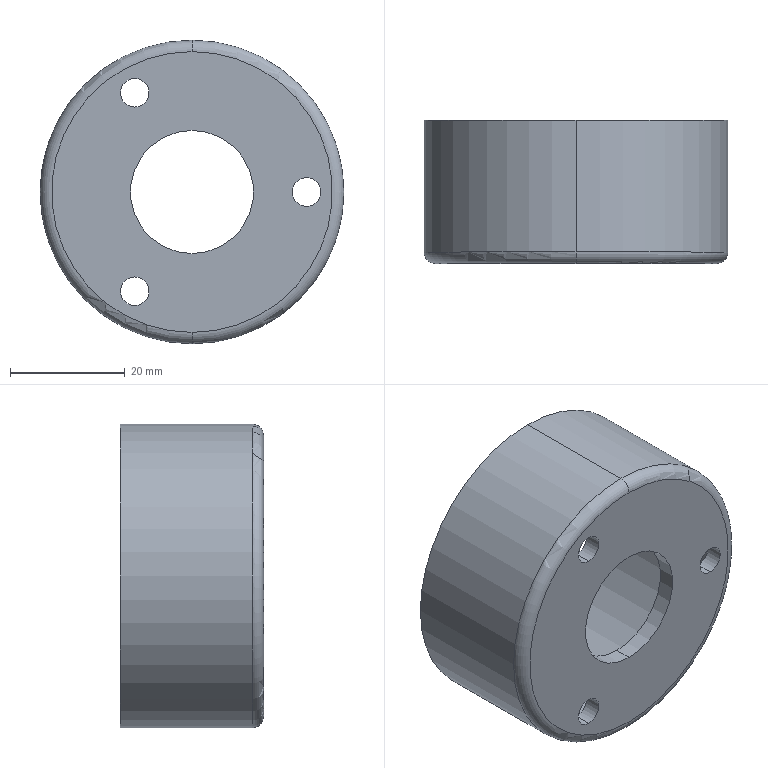Part | STEP file | 1.6米轴承套 | 1 solid | 17 faces | box 53 x 25 x 53 mm | volume 15579 mm3 | cylinder 12 | plane 3 | torus 2 | commonest cylinder face diameters 5 x6 21.5 x2 47 x2 53 x2
STEP:
#1=CARTESIAN_POINT('',(0.,0.,-10.75));
#2=VERTEX_POINT('',#1);
#3=CARTESIAN_POINT('',(0.,0.,10.75));
#4=VERTEX_POINT('',#3);
#5=CARTESIAN_POINT('',(0.,0.,0.));
#6=DIRECTION('',(0.,1.,0.));
#7=DIRECTION('',(0.,0.,1.));
#8=AXIS2_PLACEMENT_3D('',#5,#6,#7);
#9=CIRCLE('',#8,10.75);
#10=EDGE_CURVE('',#2,#4,#9,.T.);
#11=ORIENTED_EDGE('',*,*,#10,.F.);
#12=CARTESIAN_POINT('',(0.,3.,-10.75));
#13=VERTEX_POINT('',#12);
#14=CARTESIAN_POINT('',(0.,-22.,-10.75));
#15=DIRECTION('',(0.,1.,0.));
#16=VECTOR('',#15,1000.);
#17=LINE('',#14,#16);
#18=EDGE_CURVE('',#2,#13,#17,.T.);
#19=ORIENTED_EDGE('',*,*,#18,.T.);
#20=CARTESIAN_POINT('',(0.,3.,10.75));
#21=VERTEX_POINT('',#20);
#22=CARTESIAN_POINT('',(0.,3.,0.));
#23=DIRECTION('',(0.,1.,0.));
#24=DIRECTION('',(0.,0.,1.));
#25=AXIS2_PLACEMENT_3D('',#22,#23,#24);
#26=CIRCLE('',#25,10.75);
#27=EDGE_CURVE('',#13,#21,#26,.T.);
#28=ORIENTED_EDGE('',*,*,#27,.T.);
#29=CARTESIAN_POINT('',(0.,-22.,10.75));
#30=DIRECTION('',(0.,1.,0.));
#31=VECTOR('',#30,1000.);
#32=LINE('',#29,#31);
#33=EDGE_CURVE('',#4,#21,#32,.T.);
#34=ORIENTED_EDGE('',*,*,#33,.F.);
#35=EDGE_LOOP('',(#11,#19,#28,#34));
#36=FACE_OUTER_BOUND('',#35,.T.);
#37=CARTESIAN_POINT('',(0.,-22.,0.));
#38=DIRECTION('',(0.,1.,0.));
#39=DIRECTION('',(0.,0.,1.));
#40=AXIS2_PLACEMENT_3D('',#37,#38,#39);
#41=CYLINDRICAL_SURFACE('',#40,10.75);
#42=ADVANCED_FACE('',(#36),#41,.F.);
#43=CARTESIAN_POINT('',(20.,0.,-2.5));
#44=VERTEX_POINT('',#43);
#45=CARTESIAN_POINT('',(20.,0.,2.5));
#46=VERTEX_POINT('',#45);
#47=CARTESIAN_POINT('',(20.,0.,0.));
#48=DIRECTION('',(0.,1.,0.));
#49=DIRECTION('',(0.,0.,1.));
#50=AXIS2_PLACEMENT_3D('',#47,#48,#49);
#51=CIRCLE('',#50,2.5);
#52=EDGE_CURVE('',#44,#46,#51,.T.);
#53=ORIENTED_EDGE('',*,*,#52,.F.);
#54=CARTESIAN_POINT('',(20.,3.,-2.5));
#55=VERTEX_POINT('',#54);
#56=CARTESIAN_POINT('',(20.,3.,-2.5));
#57=DIRECTION('',(0.,1.,0.));
#58=VECTOR('',#57,1000.);
#59=LINE('',#56,#58);
#60=EDGE_CURVE('',#44,#55,#59,.T.);
#61=ORIENTED_EDGE('',*,*,#60,.T.);
#62=CARTESIAN_POINT('',(20.,3.,2.5));
#63=VERTEX_POINT('',#62);
#64=CARTESIAN_POINT('',(20.,3.,0.));
#65=DIRECTION('',(0.,1.,0.));
#66=DIRECTION('',(0.,0.,1.));
#67=AXIS2_PLACEMENT_3D('',#64,#65,#66);
#68=CIRCLE('',#67,2.5);
#69=EDGE_CURVE('',#55,#63,#68,.T.);
#70=ORIENTED_EDGE('',*,*,#69,.T.);
#71=CARTESIAN_POINT('',(20.,3.,2.5));
#72=DIRECTION('',(0.,1.,0.));
#73=VECTOR('',#72,1000.);
#74=LINE('',#71,#73);
#75=EDGE_CURVE('',#46,#63,#74,.T.);
#76=ORIENTED_EDGE('',*,*,#75,.F.);
#77=EDGE_LOOP('',(#53,#61,#70,#76));
#78=FACE_OUTER_BOUND('',#77,.T.);
#79=CARTESIAN_POINT('',(20.,3.,0.));
#80=DIRECTION('',(0.,1.,0.));
#81=DIRECTION('',(0.,0.,1.));
#82=AXIS2_PLACEMENT_3D('',#79,#80,#81);
#83=CYLINDRICAL_SURFACE('',#82,2.5);
#84=ADVANCED_FACE('',(#78),#83,.F.);
#85=CARTESIAN_POINT('',(-10.,0.,14.821));
#86=VERTEX_POINT('',#85);
#87=CARTESIAN_POINT('',(-10.,0.,19.821));
#88=VERTEX_POINT('',#87);
#89=CARTESIAN_POINT('',(-10.,0.,17.321));
#90=DIRECTION('',(0.,1.,0.));
#91=DIRECTION('',(0.,0.,1.));
#92=AXIS2_PLACEMENT_3D('',#89,#90,#91);
#93=CIRCLE('',#92,2.5);
#94=EDGE_CURVE('',#86,#88,#93,.T.);
#95=ORIENTED_EDGE('',*,*,#94,.F.);
#96=CARTESIAN_POINT('',(-10.,3.,14.821));
#97=VERTEX_POINT('',#96);
#98=CARTESIAN_POINT('',(-10.,3.,14.821));
#99=DIRECTION('',(0.,1.,0.));
#100=VECTOR('',#99,1000.);
#101=LINE('',#98,#100);
#102=EDGE_CURVE('',#86,#97,#101,.T.);
#103=ORIENTED_EDGE('',*,*,#102,.T.);
#104=CARTESIAN_POINT('',(-10.,3.,19.821));
#105=VERTEX_POINT('',#104);
#106=CARTESIAN_POINT('',(-10.,3.,17.321));
#107=DIRECTION('',(0.,1.,0.));
#108=DIRECTION('',(0.,0.,1.));
#109=AXIS2_PLACEMENT_3D('',#106,#107,#108);
#110=CIRCLE('',#109,2.5);
#111=EDGE_CURVE('',#97,#105,#110,.T.);
#112=ORIENTED_EDGE('',*,*,#111,.T.);
#113=CARTESIAN_POINT('',(-10.,3.,19.821));
#114=DIRECTION('',(0.,1.,0.));
#115=VECTOR('',#114,1000.);
#116=LINE('',#113,#115);
#117=EDGE_CURVE('',#88,#105,#116,.T.);
#118=ORIENTED_EDGE('',*,*,#117,.F.);
#119=EDGE_LOOP('',(#95,#103,#112,#118));
#120=FACE_OUTER_BOUND('',#119,.T.);
#121=CARTESIAN_POINT('',(-10.,3.,17.321));
#122=DIRECTION('',(0.,1.,0.));
#123=DIRECTION('',(0.,0.,1.));
#124=AXIS2_PLACEMENT_3D('',#121,#122,#123);
#125=CYLINDRICAL_SURFACE('',#124,2.5);
#126=ADVANCED_FACE('',(#120),#125,.F.);
#127=CARTESIAN_POINT('',(-10.,0.,-19.821));
#128=VERTEX_POINT('',#127);
#129=CARTESIAN_POINT('',(-10.,0.,-14.821));
#130=VERTEX_POINT('',#129);
#131=CARTESIAN_POINT('',(-10.,0.,-17.321));
#132=DIRECTION('',(0.,1.,0.));
#133=DIRECTION('',(0.,0.,1.));
#134=AXIS2_PLACEMENT_3D('',#131,#132,#133);
#135=CIRCLE('',#134,2.5);
#136=EDGE_CURVE('',#128,#130,#135,.T.);
#137=ORIENTED_EDGE('',*,*,#136,.F.);
#138=CARTESIAN_POINT('',(-10.,3.,-19.821));
#139=VERTEX_POINT('',#138);
#140=CARTESIAN_POINT('',(-10.,3.,-19.821));
#141=DIRECTION('',(0.,1.,0.));
#142=VECTOR('',#141,1000.);
#143=LINE('',#140,#142);
#144=EDGE_CURVE('',#128,#139,#143,.T.);
#145=ORIENTED_EDGE('',*,*,#144,.T.);
#146=CARTESIAN_POINT('',(-10.,3.,-14.821));
#147=VERTEX_POINT('',#146);
#148=CARTESIAN_POINT('',(-10.,3.,-17.321));
#149=DIRECTION('',(0.,1.,0.));
#150=DIRECTION('',(0.,0.,1.));
#151=AXIS2_PLACEMENT_3D('',#148,#149,#150);
#152=CIRCLE('',#151,2.5);
#153=EDGE_CURVE('',#139,#147,#152,.T.);
#154=ORIENTED_EDGE('',*,*,#153,.T.);
#155=CARTESIAN_POINT('',(-10.,3.,-14.821));
#156=DIRECTION('',(0.,1.,0.));
#157=VECTOR('',#156,1000.);
#158=LINE('',#155,#157);
#159=EDGE_CURVE('',#130,#147,#158,.T.);
#160=ORIENTED_EDGE('',*,*,#159,.F.);
#161=EDGE_LOOP('',(#137,#145,#154,#160));
#162=FACE_OUTER_BOUND('',#161,.T.);
#163=CARTESIAN_POINT('',(-10.,3.,-17.321));
#164=DIRECTION('',(0.,1.,0.));
#165=DIRECTION('',(0.,0.,1.));
#166=AXIS2_PLACEMENT_3D('',#163,#164,#165);
#167=CYLINDRICAL_SURFACE('',#166,2.5);
#168=ADVANCED_FACE('',(#162),#167,.F.);
#169=CARTESIAN_POINT('',(0.,0.,-24.5));
#170=VERTEX_POINT('',#169);
#171=CARTESIAN_POINT('',(0.,0.,24.5));
#172=VERTEX_POINT('',#171);
#173=CARTESIAN_POINT('',(0.,0.,0.));
#174=DIRECTION('',(0.,-1.,0.));
#175=DIRECTION('',(0.,0.,1.));
#176=AXIS2_PLACEMENT_3D('',#173,#174,#175);
#177=CIRCLE('',#176,24.5);
#178=EDGE_CURVE('',#170,#172,#177,.T.);
#179=ORIENTED_EDGE('',*,*,#178,.F.);
#180=CARTESIAN_POINT('',(0.,2.,-26.5));
#181=VERTEX_POINT('',#180);
#182=CARTESIAN_POINT('',(0.,2.,-24.5));
#183=DIRECTION('',(1.,0.,0.));
#184=DIRECTION('',(0.,0.,-1.));
#185=AXIS2_PLACEMENT_3D('',#182,#183,#184);
#186=CIRCLE('',#185,2.);
#187=EDGE_CURVE('',#170,#181,#186,.T.);
#188=ORIENTED_EDGE('',*,*,#187,.T.);
#189=CARTESIAN_POINT('',(0.,2.,26.5));
#190=VERTEX_POINT('',#189);
#191=CARTESIAN_POINT('',(0.,2.,0.));
#192=DIRECTION('',(0.,1.,0.));
#193=DIRECTION('',(0.,0.,1.));
#194=AXIS2_PLACEMENT_3D('',#191,#192,#193);
#195=CIRCLE('',#194,26.5);
#196=EDGE_CURVE('',#190,#181,#195,.T.);
#197=ORIENTED_EDGE('',*,*,#196,.F.);
#198=CARTESIAN_POINT('',(0.,2.,24.5));
#199=DIRECTION('',(-1.,0.,0.));
#200=DIRECTION('',(0.,0.,1.));
#201=AXIS2_PLACEMENT_3D('',#198,#199,#200);
#202=CIRCLE('',#201,2.);
#203=EDGE_CURVE('',#172,#190,#202,.T.);
#204=ORIENTED_EDGE('',*,*,#203,.F.);
#205=EDGE_LOOP('',(#179,#188,#197,#204));
#206=FACE_OUTER_BOUND('',#205,.T.);
#207=CARTESIAN_POINT('',(0.,2.,0.));
#208=DIRECTION('',(0.,1.,0.));
#209=DIRECTION('',(0.,0.,1.));
#210=AXIS2_PLACEMENT_3D('',#207,#208,#209);
#211=TOROIDAL_SURFACE('',#210,24.5,2.);
#212=ADVANCED_FACE('',(#206),#211,.T.);
#213=CARTESIAN_POINT('',(0.,25.,-23.5));
#214=VERTEX_POINT('',#213);
#215=CARTESIAN_POINT('',(0.,25.,23.5));
#216=VERTEX_POINT('',#215);
#217=CARTESIAN_POINT('',(0.,25.,0.));
#218=DIRECTION('',(0.,1.,0.));
#219=DIRECTION('',(0.,0.,1.));
#220=AXIS2_PLACEMENT_3D('',#217,#218,#219);
#221=CIRCLE('',#220,23.5);
#222=EDGE_CURVE('',#214,#216,#221,.T.);
#223=ORIENTED_EDGE('',*,*,#222,.T.);
#224=CARTESIAN_POINT('',(0.,3.,23.5));
#225=VERTEX_POINT('',#224);
#226=CARTESIAN_POINT('',(0.,25.,23.5));
#227=DIRECTION('',(0.,-1.,0.));
#228=VECTOR('',#227,1000.);
#229=LINE('',#226,#228);
#230=EDGE_CURVE('',#216,#225,#229,.T.);
#231=ORIENTED_EDGE('',*,*,#230,.T.);
#232=CARTESIAN_POINT('',(0.,3.,-23.5));
#233=VERTEX_POINT('',#232);
#234=CARTESIAN_POINT('',(0.,3.,0.));
#235=DIRECTION('',(0.,1.,0.));
#236=DIRECTION('',(0.,0.,1.));
#237=AXIS2_PLACEMENT_3D('',#234,#235,#236);
#238=CIRCLE('',#237,23.5);
#239=EDGE_CURVE('',#233,#225,#238,.T.);
#240=ORIENTED_EDGE('',*,*,#239,.F.);
#241=CARTESIAN_POINT('',(0.,25.,-23.5));
#242=DIRECTION('',(0.,-1.,0.));
#243=VECTOR('',#242,1000.);
#244=LINE('',#241,#243);
#245=EDGE_CURVE('',#214,#233,#244,.T.);
#246=ORIENTED_EDGE('',*,*,#245,.F.);
#247=EDGE_LOOP('',(#223,#231,#240,#246));
#248=FACE_OUTER_BOUND('',#247,.T.);
#249=CARTESIAN_POINT('',(0.,25.,0.));
#250=DIRECTION('',(0.,-1.,0.));
#251=DIRECTION('',(0.,0.,-1.));
#252=AXIS2_PLACEMENT_3D('',#249,#250,#251);
#253=CYLINDRICAL_SURFACE('',#252,23.5);
#254=ADVANCED_FACE('',(#248),#253,.F.);
#255=CARTESIAN_POINT('',(0.,25.,26.5));
#256=VERTEX_POINT('',#255);
#257=CARTESIAN_POINT('',(0.,25.,-26.5));
#258=VERTEX_POINT('',#257);
#259=CARTESIAN_POINT('',(0.,25.,0.));
#260=DIRECTION('',(0.,1.,0.));
#261=DIRECTION('',(0.,0.,1.));
#262=AXIS2_PLACEMENT_3D('',#259,#260,#261);
#263=CIRCLE('',#262,26.5);
#264=EDGE_CURVE('',#256,#258,#263,.T.);
#265=ORIENTED_EDGE('',*,*,#264,.F.);
#266=CARTESIAN_POINT('',(0.,25.,26.5));
#267=DIRECTION('',(0.,-1.,0.));
#268=VECTOR('',#267,1000.);
#269=LINE('',#266,#268);
#270=EDGE_CURVE('',#256,#190,#269,.T.);
#271=ORIENTED_EDGE('',*,*,#270,.T.);
#272=ORIENTED_EDGE('',*,*,#196,.T.);
#273=CARTESIAN_POINT('',(0.,25.,-26.5));
#274=DIRECTION('',(0.,-1.,0.));
#275=VECTOR('',#274,1000.);
#276=LINE('',#273,#275);
#277=EDGE_CURVE('',#258,#181,#276,.T.);
#278=ORIENTED_EDGE('',*,*,#277,.F.);
#279=EDGE_LOOP('',(#265,#271,#272,#278));
#280=FACE_OUTER_BOUND('',#279,.T.);
#281=CARTESIAN_POINT('',(0.,25.,0.));
#282=DIRECTION('',(0.,-1.,0.));
#283=DIRECTION('',(0.,0.,-1.));
#284=AXIS2_PLACEMENT_3D('',#281,#282,#283);
#285=CYLINDRICAL_SURFACE('',#284,26.5);
#286=ADVANCED_FACE('',(#280),#285,.T.);
#287=ORIENTED_EDGE('',*,*,#270,.F.);
#288=CARTESIAN_POINT('',(0.,25.,0.));
#289=DIRECTION('',(0.,1.,0.));
#290=DIRECTION('',(0.,0.,1.));
#291=AXIS2_PLACEMENT_3D('',#288,#289,#290);
#292=CIRCLE('',#291,26.5);
#293=EDGE_CURVE('',#258,#256,#292,.T.);
#294=ORIENTED_EDGE('',*,*,#293,.F.);
#295=ORIENTED_EDGE('',*,*,#277,.T.);
#296=CARTESIAN_POINT('',(0.,2.,0.));
#297=DIRECTION('',(0.,1.,0.));
#298=DIRECTION('',(0.,0.,1.));
#299=AXIS2_PLACEMENT_3D('',#296,#297,#298);
#300=CIRCLE('',#299,26.5);
#301=EDGE_CURVE('',#181,#190,#300,.T.);
#302=ORIENTED_EDGE('',*,*,#301,.T.);
#303=EDGE_LOOP('',(#287,#294,#295,#302));
#304=FACE_OUTER_BOUND('',#303,.T.);
#305=CARTESIAN_POINT('',(0.,25.,0.));
#306=DIRECTION('',(0.,-1.,0.));
#307=DIRECTION('',(0.,0.,-1.));
#308=AXIS2_PLACEMENT_3D('',#305,#306,#307);
#309=CYLINDRICAL_SURFACE('',#308,26.5);
#310=ADVANCED_FACE('',(#304),#309,.T.);
#311=ORIENTED_EDGE('',*,*,#222,.F.);
#312=CARTESIAN_POINT('',(0.,25.,0.));
#313=DIRECTION('',(0.,1.,0.));
#314=DIRECTION('',(0.,0.,1.));
#315=AXIS2_PLACEMENT_3D('',#312,#313,#314);
#316=CIRCLE('',#315,23.5);
#317=EDGE_CURVE('',#216,#214,#316,.T.);
#318=ORIENTED_EDGE('',*,*,#317,.F.);
#319=EDGE_LOOP('',(#311,#318));
#320=FACE_BOUND('',#319,.T.);
#321=ORIENTED_EDGE('',*,*,#293,.T.);
#322=ORIENTED_EDGE('',*,*,#264,.T.);
#323=EDGE_LOOP('',(#321,#322));
#324=FACE_OUTER_BOUND('',#323,.T.);
#325=CARTESIAN_POINT('',(0.,25.,0.));
#326=DIRECTION('',(0.,1.,0.));
#327=DIRECTION('',(0.,0.,1.));
#328=AXIS2_PLACEMENT_3D('',#325,#326,#327);
#329=PLANE('',#328);
#330=ADVANCED_FACE('',(#320,#324),#329,.T.);
#331=CARTESIAN_POINT('',(0.,0.,0.));
#332=DIRECTION('',(0.,1.,0.));
#333=DIRECTION('',(0.,0.,1.));
#334=AXIS2_PLACEMENT_3D('',#331,#332,#333);
#335=CIRCLE('',#334,10.75);
#336=EDGE_CURVE('',#4,#2,#335,.T.);
#337=ORIENTED_EDGE('',*,*,#336,.T.);
#338=ORIENTED_EDGE('',*,*,#10,.T.);
#339=EDGE_LOOP('',(#337,#338));
#340=FACE_BOUND('',#339,.T.);
#341=CARTESIAN_POINT('',(20.,0.,0.));
#342=DIRECTION('',(0.,1.,0.));
#343=DIRECTION('',(0.,0.,1.));
#344=AXIS2_PLACEMENT_3D('',#341,#342,#343);
#345=CIRCLE('',#344,2.5);
#346=EDGE_CURVE('',#46,#44,#345,.T.);
#347=ORIENTED_EDGE('',*,*,#346,.T.);
#348=ORIENTED_EDGE('',*,*,#52,.T.);
#349=EDGE_LOOP('',(#347,#348));
#350=FACE_BOUND('',#349,.T.);
#351=CARTESIAN_POINT('',(-10.,0.,17.321));
#352=DIRECTION('',(0.,1.,0.));
#353=DIRECTION('',(0.,0.,1.));
#354=AXIS2_PLACEMENT_3D('',#351,#352,#353);
#355=CIRCLE('',#354,2.5);
#356=EDGE_CURVE('',#88,#86,#355,.T.);
#357=ORIENTED_EDGE('',*,*,#356,.T.);
#358=ORIENTED_EDGE('',*,*,#94,.T.);
#359=EDGE_LOOP('',(#357,#358));
#360=FACE_BOUND('',#359,.T.);
#361=CARTESIAN_POINT('',(-10.,0.,-17.321));
#362=DIRECTION('',(0.,1.,0.));
#363=DIRECTION('',(0.,0.,1.));
#364=AXIS2_PLACEMENT_3D('',#361,#362,#363);
#365=CIRCLE('',#364,2.5);
#366=EDGE_CURVE('',#130,#128,#365,.T.);
#367=ORIENTED_EDGE('',*,*,#366,.T.);
#368=ORIENTED_EDGE('',*,*,#136,.T.);
#369=EDGE_LOOP('',(#367,#368));
#370=FACE_BOUND('',#369,.T.);
#371=CARTESIAN_POINT('',(0.,0.,0.));
#372=DIRECTION('',(0.,-1.,0.));
#373=DIRECTION('',(0.,0.,1.));
#374=AXIS2_PLACEMENT_3D('',#371,#372,#373);
#375=CIRCLE('',#374,24.5);
#376=EDGE_CURVE('',#172,#170,#375,.T.);
#377=ORIENTED_EDGE('',*,*,#376,.T.);
#378=ORIENTED_EDGE('',*,*,#178,.T.);
#379=EDGE_LOOP('',(#377,#378));
#380=FACE_OUTER_BOUND('',#379,.T.);
#381=CARTESIAN_POINT('',(0.,0.,0.));
#382=DIRECTION('',(0.,1.,0.));
#383=DIRECTION('',(0.,0.,1.));
#384=AXIS2_PLACEMENT_3D('',#381,#382,#383);
#385=PLANE('',#384);
#386=ADVANCED_FACE('',(#340,#350,#360,#370,#380),#385,.F.);
#387=ORIENTED_EDGE('',*,*,#230,.F.);
#388=ORIENTED_EDGE('',*,*,#317,.T.);
#389=ORIENTED_EDGE('',*,*,#245,.T.);
#390=CARTESIAN_POINT('',(0.,3.,0.));
#391=DIRECTION('',(0.,1.,0.));
#392=DIRECTION('',(0.,0.,1.));
#393=AXIS2_PLACEMENT_3D('',#390,#391,#392);
#394=CIRCLE('',#393,23.5);
#395=EDGE_CURVE('',#225,#233,#394,.T.);
#396=ORIENTED_EDGE('',*,*,#395,.F.);
#397=EDGE_LOOP('',(#387,#388,#389,#396));
#398=FACE_OUTER_BOUND('',#397,.T.);
#399=CARTESIAN_POINT('',(0.,25.,0.));
#400=DIRECTION('',(0.,-1.,0.));
#401=DIRECTION('',(0.,0.,-1.));
#402=AXIS2_PLACEMENT_3D('',#399,#400,#401);
#403=CYLINDRICAL_SURFACE('',#402,23.5);
#404=ADVANCED_FACE('',(#398),#403,.F.);
#405=CARTESIAN_POINT('',(0.,3.,0.));
#406=DIRECTION('',(0.,1.,0.));
#407=DIRECTION('',(0.,0.,1.));
#408=AXIS2_PLACEMENT_3D('',#405,#406,#407);
#409=CIRCLE('',#408,10.75);
#410=EDGE_CURVE('',#21,#13,#409,.T.);
#411=ORIENTED_EDGE('',*,*,#410,.F.);
#412=ORIENTED_EDGE('',*,*,#27,.F.);
#413=EDGE_LOOP('',(#411,#412));
#414=FACE_BOUND('',#413,.T.);
#415=CARTESIAN_POINT('',(20.,3.,0.));
#416=DIRECTION('',(0.,1.,0.));
#417=DIRECTION('',(0.,0.,1.));
#418=AXIS2_PLACEMENT_3D('',#415,#416,#417);
#419=CIRCLE('',#418,2.5);
#420=EDGE_CURVE('',#63,#55,#419,.T.);
#421=ORIENTED_EDGE('',*,*,#420,.F.);
#422=ORIENTED_EDGE('',*,*,#69,.F.);
#423=EDGE_LOOP('',(#421,#422));
#424=FACE_BOUND('',#423,.T.);
#425=CARTESIAN_POINT('',(-10.,3.,17.321));
#426=DIRECTION('',(0.,1.,0.));
#427=DIRECTION('',(0.,0.,1.));
#428=AXIS2_PLACEMENT_3D('',#425,#426,#427);
#429=CIRCLE('',#428,2.5);
#430=EDGE_CURVE('',#105,#97,#429,.T.);
#431=ORIENTED_EDGE('',*,*,#430,.F.);
#432=ORIENTED_EDGE('',*,*,#111,.F.);
#433=EDGE_LOOP('',(#431,#432));
#434=FACE_BOUND('',#433,.T.);
#435=CARTESIAN_POINT('',(-10.,3.,-17.321));
#436=DIRECTION('',(0.,1.,0.));
#437=DIRECTION('',(0.,0.,1.));
#438=AXIS2_PLACEMENT_3D('',#435,#436,#437);
#439=CIRCLE('',#438,2.5);
#440=EDGE_CURVE('',#147,#139,#439,.T.);
#441=ORIENTED_EDGE('',*,*,#440,.F.);
#442=ORIENTED_EDGE('',*,*,#153,.F.);
#443=EDGE_LOOP('',(#441,#442));
#444=FACE_BOUND('',#443,.T.);
#445=ORIENTED_EDGE('',*,*,#239,.T.);
#446=ORIENTED_EDGE('',*,*,#395,.T.);
#447=EDGE_LOOP('',(#445,#446));
#448=FACE_OUTER_BOUND('',#447,.T.);
#449=CARTESIAN_POINT('',(0.,3.,0.));
#450=DIRECTION('',(0.,1.,0.));
#451=DIRECTION('',(0.,0.,1.));
#452=AXIS2_PLACEMENT_3D('',#449,#450,#451);
#453=PLANE('',#452);
#454=ADVANCED_FACE('',(#414,#424,#434,#444,#448),#453,.T.);
#455=ORIENTED_EDGE('',*,*,#187,.F.);
#456=ORIENTED_EDGE('',*,*,#376,.F.);
#457=ORIENTED_EDGE('',*,*,#203,.T.);
#458=ORIENTED_EDGE('',*,*,#301,.F.);
#459=EDGE_LOOP('',(#455,#456,#457,#458));
#460=FACE_OUTER_BOUND('',#459,.T.);
#461=CARTESIAN_POINT('',(0.,2.,0.));
#462=DIRECTION('',(0.,1.,0.));
#463=DIRECTION('',(0.,0.,1.));
#464=AXIS2_PLACEMENT_3D('',#461,#462,#463);
#465=TOROIDAL_SURFACE('',#464,24.5,2.);
#466=ADVANCED_FACE('',(#460),#465,.T.);
#467=ORIENTED_EDGE('',*,*,#144,.F.);
#468=ORIENTED_EDGE('',*,*,#366,.F.);
#469=ORIENTED_EDGE('',*,*,#159,.T.);
#470=ORIENTED_EDGE('',*,*,#440,.T.);
#471=EDGE_LOOP('',(#467,#468,#469,#470));
#472=FACE_OUTER_BOUND('',#471,.T.);
#473=CARTESIAN_POINT('',(-10.,3.,-17.321));
#474=DIRECTION('',(0.,1.,0.));
#475=DIRECTION('',(0.,0.,1.));
#476=AXIS2_PLACEMENT_3D('',#473,#474,#475);
#477=CYLINDRICAL_SURFACE('',#476,2.5);
#478=ADVANCED_FACE('',(#472),#477,.F.);
#479=ORIENTED_EDGE('',*,*,#102,.F.);
#480=ORIENTED_EDGE('',*,*,#356,.F.);
#481=ORIENTED_EDGE('',*,*,#117,.T.);
#482=ORIENTED_EDGE('',*,*,#430,.T.);
#483=EDGE_LOOP('',(#479,#480,#481,#482));
#484=FACE_OUTER_BOUND('',#483,.T.);
#485=CARTESIAN_POINT('',(-10.,3.,17.321));
#486=DIRECTION('',(0.,1.,0.));
#487=DIRECTION('',(0.,0.,1.));
#488=AXIS2_PLACEMENT_3D('',#485,#486,#487);
#489=CYLINDRICAL_SURFACE('',#488,2.5);
#490=ADVANCED_FACE('',(#484),#489,.F.);
#491=ORIENTED_EDGE('',*,*,#60,.F.);
#492=ORIENTED_EDGE('',*,*,#346,.F.);
#493=ORIENTED_EDGE('',*,*,#75,.T.);
#494=ORIENTED_EDGE('',*,*,#420,.T.);
#495=EDGE_LOOP('',(#491,#492,#493,#494));
#496=FACE_OUTER_BOUND('',#495,.T.);
#497=CARTESIAN_POINT('',(20.,3.,0.));
#498=DIRECTION('',(0.,1.,0.));
#499=DIRECTION('',(0.,0.,1.));
#500=AXIS2_PLACEMENT_3D('',#497,#498,#499);
#501=CYLINDRICAL_SURFACE('',#500,2.5);
#502=ADVANCED_FACE('',(#496),#501,.F.);
#503=ORIENTED_EDGE('',*,*,#18,.F.);
#504=ORIENTED_EDGE('',*,*,#336,.F.);
#505=ORIENTED_EDGE('',*,*,#33,.T.);
#506=ORIENTED_EDGE('',*,*,#410,.T.);
#507=EDGE_LOOP('',(#503,#504,#505,#506));
#508=FACE_OUTER_BOUND('',#507,.T.);
#509=CARTESIAN_POINT('',(0.,-22.,0.));
#510=DIRECTION('',(0.,1.,0.));
#511=DIRECTION('',(0.,0.,1.));
#512=AXIS2_PLACEMENT_3D('',#509,#510,#511);
#513=CYLINDRICAL_SURFACE('',#512,10.75);
#514=ADVANCED_FACE('',(#508),#513,.F.);
#515=CLOSED_SHELL('',(#42,#84,#126,#168,#212,#254,#286,#310,#330,#386,#404,#454,#466,#478,#490,#502,#514));
#516=MANIFOLD_SOLID_BREP('',#515);
#517=CARTESIAN_POINT('',(0.,0.,0.));
#518=DIRECTION('',(0.,0.,1.));
#519=DIRECTION('',(1.,0.,0.));
#520=AXIS2_PLACEMENT_3D('',#517,#518,#519);
#521=(LENGTH_UNIT()NAMED_UNIT(*)SI_UNIT(.MILLI.,.METRE.));
#522=UNCERTAINTY_MEASURE_WITH_UNIT(LENGTH_MEASURE(0.00001),#521,'','');
#523=(NAMED_UNIT(*)PLANE_ANGLE_UNIT()SI_UNIT($,.RADIAN.));
#524=(NAMED_UNIT(*)SI_UNIT($,.STERADIAN.)SOLID_ANGLE_UNIT());
#525=(GEOMETRIC_REPRESENTATION_CONTEXT(3)GLOBAL_UNCERTAINTY_ASSIGNED_CONTEXT((#522))GLOBAL_UNIT_ASSIGNED_CONTEXT((#521,#523,#524))REPRESENTATION_CONTEXT('',''));
#526=ADVANCED_BREP_SHAPE_REPRESENTATION('',(#516,#520),#525);